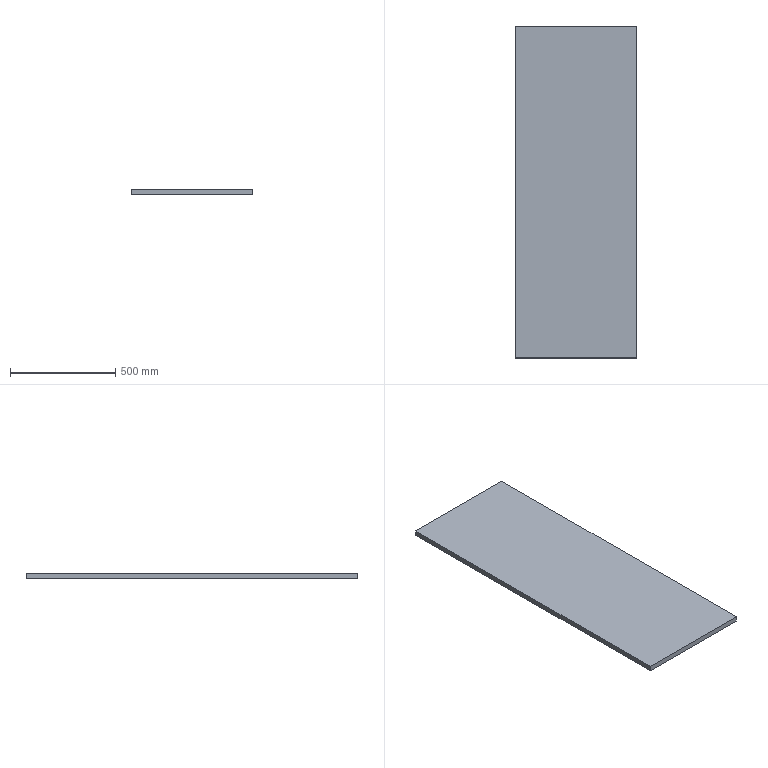Part | SolidWorks | features Extrusion 1, ICE 1 | 1 solid | 6 faces | box 580 x 1580 x 25 mm | volume 22910000 mm3 | plane 6
STEP:
#1=CARTESIAN_POINT('',(290.,-790.,0.));
#2=VERTEX_POINT('',#1);
#3=CARTESIAN_POINT('',(290.,790.,0.));
#4=VERTEX_POINT('',#3);
#5=CARTESIAN_POINT('',(290.,-790.,0.));
#6=DIRECTION('',(0.,1.,0.));
#7=VECTOR('',#6,1000.);
#8=LINE('',#5,#7);
#9=EDGE_CURVE('',#2,#4,#8,.T.);
#10=ORIENTED_EDGE('',*,*,#9,.F.);
#11=CARTESIAN_POINT('',(-290.,-790.,0.));
#12=VERTEX_POINT('',#11);
#13=CARTESIAN_POINT('',(-290.,-790.,0.));
#14=DIRECTION('',(1.,0.,0.));
#15=VECTOR('',#14,1000.);
#16=LINE('',#13,#15);
#17=EDGE_CURVE('',#12,#2,#16,.T.);
#18=ORIENTED_EDGE('',*,*,#17,.F.);
#19=CARTESIAN_POINT('',(-290.,790.,0.));
#20=VERTEX_POINT('',#19);
#21=CARTESIAN_POINT('',(-290.,-790.,0.));
#22=DIRECTION('',(0.,-1.,0.));
#23=VECTOR('',#22,1000.);
#24=LINE('',#21,#23);
#25=EDGE_CURVE('',#20,#12,#24,.T.);
#26=ORIENTED_EDGE('',*,*,#25,.F.);
#27=CARTESIAN_POINT('',(-290.,790.,0.));
#28=DIRECTION('',(-1.,0.,0.));
#29=VECTOR('',#28,1000.);
#30=LINE('',#27,#29);
#31=EDGE_CURVE('',#4,#20,#30,.T.);
#32=ORIENTED_EDGE('',*,*,#31,.F.);
#33=EDGE_LOOP('',(#10,#18,#26,#32));
#34=FACE_OUTER_BOUND('',#33,.T.);
#35=CARTESIAN_POINT('',(0.,0.,0.));
#36=DIRECTION('',(0.,0.,1.));
#37=DIRECTION('',(1.,0.,0.));
#38=AXIS2_PLACEMENT_3D('',#35,#36,#37);
#39=PLANE('',#38);
#40=ADVANCED_FACE('',(#34),#39,.F.);
#41=CARTESIAN_POINT('',(290.,-790.,25.));
#42=VERTEX_POINT('',#41);
#43=CARTESIAN_POINT('',(290.,790.,25.));
#44=VERTEX_POINT('',#43);
#45=CARTESIAN_POINT('',(290.,-790.,25.));
#46=DIRECTION('',(0.,1.,0.));
#47=VECTOR('',#46,1000.);
#48=LINE('',#45,#47);
#49=EDGE_CURVE('',#42,#44,#48,.T.);
#50=ORIENTED_EDGE('',*,*,#49,.F.);
#51=CARTESIAN_POINT('',(290.,-790.,0.));
#52=DIRECTION('',(0.,0.,1.));
#53=VECTOR('',#52,1000.);
#54=LINE('',#51,#53);
#55=EDGE_CURVE('',#2,#42,#54,.T.);
#56=ORIENTED_EDGE('',*,*,#55,.F.);
#57=ORIENTED_EDGE('',*,*,#9,.T.);
#58=CARTESIAN_POINT('',(290.,790.,0.));
#59=DIRECTION('',(0.,0.,1.));
#60=VECTOR('',#59,1000.);
#61=LINE('',#58,#60);
#62=EDGE_CURVE('',#4,#44,#61,.T.);
#63=ORIENTED_EDGE('',*,*,#62,.T.);
#64=EDGE_LOOP('',(#50,#56,#57,#63));
#65=FACE_OUTER_BOUND('',#64,.T.);
#66=CARTESIAN_POINT('',(290.,-790.,0.));
#67=DIRECTION('',(1.,0.,0.));
#68=DIRECTION('',(0.,0.,-1.));
#69=AXIS2_PLACEMENT_3D('',#66,#67,#68);
#70=PLANE('',#69);
#71=ADVANCED_FACE('',(#65),#70,.T.);
#72=CARTESIAN_POINT('',(-290.,-790.,25.));
#73=VERTEX_POINT('',#72);
#74=CARTESIAN_POINT('',(-290.,-790.,25.));
#75=DIRECTION('',(1.,0.,0.));
#76=VECTOR('',#75,1000.);
#77=LINE('',#74,#76);
#78=EDGE_CURVE('',#73,#42,#77,.T.);
#79=ORIENTED_EDGE('',*,*,#78,.F.);
#80=CARTESIAN_POINT('',(-290.,-790.,0.));
#81=DIRECTION('',(0.,0.,1.));
#82=VECTOR('',#81,1000.);
#83=LINE('',#80,#82);
#84=EDGE_CURVE('',#12,#73,#83,.T.);
#85=ORIENTED_EDGE('',*,*,#84,.F.);
#86=ORIENTED_EDGE('',*,*,#17,.T.);
#87=ORIENTED_EDGE('',*,*,#55,.T.);
#88=EDGE_LOOP('',(#79,#85,#86,#87));
#89=FACE_OUTER_BOUND('',#88,.T.);
#90=CARTESIAN_POINT('',(-290.,-790.,0.));
#91=DIRECTION('',(0.,-1.,0.));
#92=DIRECTION('',(0.,0.,-1.));
#93=AXIS2_PLACEMENT_3D('',#90,#91,#92);
#94=PLANE('',#93);
#95=ADVANCED_FACE('',(#89),#94,.T.);
#96=CARTESIAN_POINT('',(-290.,790.,25.));
#97=VERTEX_POINT('',#96);
#98=CARTESIAN_POINT('',(-290.,-790.,25.));
#99=DIRECTION('',(0.,-1.,0.));
#100=VECTOR('',#99,1000.);
#101=LINE('',#98,#100);
#102=EDGE_CURVE('',#97,#73,#101,.T.);
#103=ORIENTED_EDGE('',*,*,#102,.F.);
#104=CARTESIAN_POINT('',(-290.,790.,0.));
#105=DIRECTION('',(0.,0.,1.));
#106=VECTOR('',#105,1000.);
#107=LINE('',#104,#106);
#108=EDGE_CURVE('',#20,#97,#107,.T.);
#109=ORIENTED_EDGE('',*,*,#108,.F.);
#110=ORIENTED_EDGE('',*,*,#25,.T.);
#111=ORIENTED_EDGE('',*,*,#84,.T.);
#112=EDGE_LOOP('',(#103,#109,#110,#111));
#113=FACE_OUTER_BOUND('',#112,.T.);
#114=CARTESIAN_POINT('',(-290.,-790.,0.));
#115=DIRECTION('',(-1.,0.,0.));
#116=DIRECTION('',(0.,0.,1.));
#117=AXIS2_PLACEMENT_3D('',#114,#115,#116);
#118=PLANE('',#117);
#119=ADVANCED_FACE('',(#113),#118,.T.);
#120=CARTESIAN_POINT('',(-290.,790.,25.));
#121=DIRECTION('',(-1.,0.,0.));
#122=VECTOR('',#121,1000.);
#123=LINE('',#120,#122);
#124=EDGE_CURVE('',#44,#97,#123,.T.);
#125=ORIENTED_EDGE('',*,*,#124,.F.);
#126=ORIENTED_EDGE('',*,*,#62,.F.);
#127=ORIENTED_EDGE('',*,*,#31,.T.);
#128=ORIENTED_EDGE('',*,*,#108,.T.);
#129=EDGE_LOOP('',(#125,#126,#127,#128));
#130=FACE_OUTER_BOUND('',#129,.T.);
#131=CARTESIAN_POINT('',(-290.,790.,0.));
#132=DIRECTION('',(0.,1.,0.));
#133=DIRECTION('',(0.,0.,1.));
#134=AXIS2_PLACEMENT_3D('',#131,#132,#133);
#135=PLANE('',#134);
#136=ADVANCED_FACE('',(#130),#135,.T.);
#137=ORIENTED_EDGE('',*,*,#78,.T.);
#138=ORIENTED_EDGE('',*,*,#49,.T.);
#139=ORIENTED_EDGE('',*,*,#124,.T.);
#140=ORIENTED_EDGE('',*,*,#102,.T.);
#141=EDGE_LOOP('',(#137,#138,#139,#140));
#142=FACE_OUTER_BOUND('',#141,.T.);
#143=CARTESIAN_POINT('',(0.,0.,25.));
#144=DIRECTION('',(0.,0.,1.));
#145=DIRECTION('',(1.,0.,0.));
#146=AXIS2_PLACEMENT_3D('',#143,#144,#145);
#147=PLANE('',#146);
#148=ADVANCED_FACE('',(#142),#147,.T.);
#149=CLOSED_SHELL('',(#40,#71,#95,#119,#136,#148));
#150=MANIFOLD_SOLID_BREP('',#149);
#151=CARTESIAN_POINT('',(0.,0.,0.));
#152=DIRECTION('',(0.,0.,1.));
#153=DIRECTION('',(1.,0.,0.));
#154=AXIS2_PLACEMENT_3D('',#151,#152,#153);
#155=(LENGTH_UNIT()NAMED_UNIT(*)SI_UNIT(.MILLI.,.METRE.));
#156=UNCERTAINTY_MEASURE_WITH_UNIT(LENGTH_MEASURE(0.00001),#155,'','');
#157=(NAMED_UNIT(*)PLANE_ANGLE_UNIT()SI_UNIT($,.RADIAN.));
#158=(NAMED_UNIT(*)SI_UNIT($,.STERADIAN.)SOLID_ANGLE_UNIT());
#159=(GEOMETRIC_REPRESENTATION_CONTEXT(3)GLOBAL_UNCERTAINTY_ASSIGNED_CONTEXT((#156))GLOBAL_UNIT_ASSIGNED_CONTEXT((#155,#157,#158))REPRESENTATION_CONTEXT('',''));
#160=ADVANCED_BREP_SHAPE_REPRESENTATION('',(#150,#154),#159);